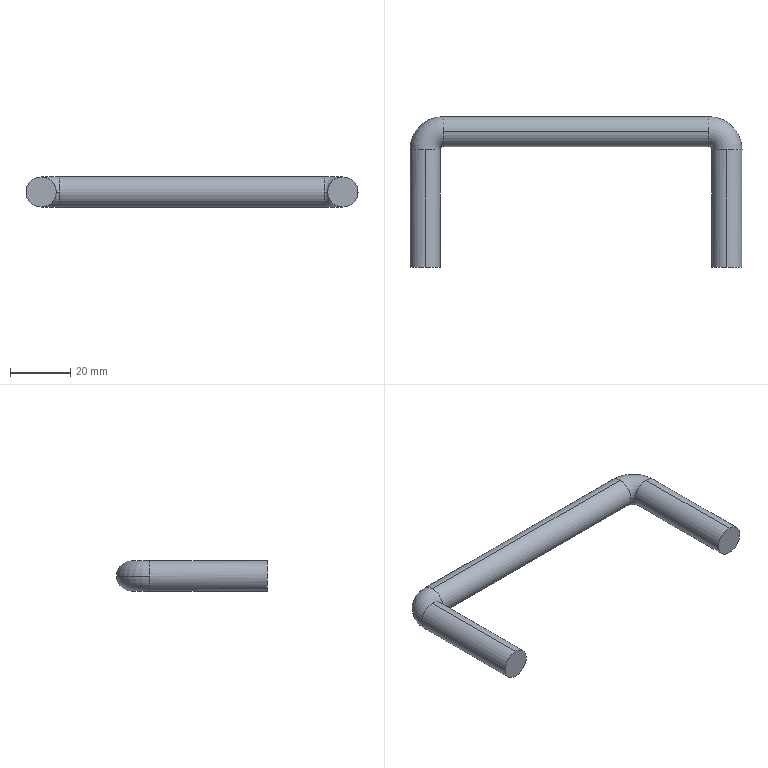Part | SolidWorks | features Sweep 1 | 1 solid | 12 faces | box 110 x 50 x 10 mm | volume 14518 mm3 | cylinder 6 | torus 4 | plane 2 | commonest cylinder face diameters 10 x6
STEP:
#1=CARTESIAN_POINT('',(-15.998,28.558,-5.));
#2=VERTEX_POINT('',#1);
#3=CARTESIAN_POINT('',(-20.998,28.558,0.));
#4=VERTEX_POINT('',#3);
#5=CARTESIAN_POINT('',(-15.998,28.558,0.));
#6=DIRECTION('',(0.,1.,0.));
#7=DIRECTION('',(0.,0.,1.));
#8=AXIS2_PLACEMENT_3D('',#5,#6,#7);
#9=CIRCLE('',#8,5.);
#10=EDGE_CURVE('',#2,#4,#9,.T.);
#11=ORIENTED_EDGE('',*,*,#10,.T.);
#12=CARTESIAN_POINT('',(-9.998,39.558,0.));
#13=VERTEX_POINT('',#12);
#14=CARTESIAN_POINT('',(-9.998,28.558,0.));
#15=DIRECTION('',(0.,0.,-1.));
#16=DIRECTION('',(-1.,0.,0.));
#17=AXIS2_PLACEMENT_3D('',#14,#15,#16);
#18=CIRCLE('',#17,11.);
#19=EDGE_CURVE('',#4,#13,#18,.T.);
#20=ORIENTED_EDGE('',*,*,#19,.T.);
#21=CARTESIAN_POINT('',(-9.998,34.558,-5.));
#22=VERTEX_POINT('',#21);
#23=CARTESIAN_POINT('',(-9.998,34.558,0.));
#24=DIRECTION('',(1.,0.,0.));
#25=DIRECTION('',(0.,0.,1.));
#26=AXIS2_PLACEMENT_3D('',#23,#24,#25);
#27=CIRCLE('',#26,5.);
#28=EDGE_CURVE('',#22,#13,#27,.T.);
#29=ORIENTED_EDGE('',*,*,#28,.F.);
#30=CARTESIAN_POINT('',(-9.998,29.558,0.));
#31=VERTEX_POINT('',#30);
#32=CARTESIAN_POINT('',(-9.998,34.558,0.));
#33=DIRECTION('',(1.,0.,0.));
#34=DIRECTION('',(0.,0.,1.));
#35=AXIS2_PLACEMENT_3D('',#32,#33,#34);
#36=CIRCLE('',#35,5.);
#37=EDGE_CURVE('',#31,#22,#36,.T.);
#38=ORIENTED_EDGE('',*,*,#37,.F.);
#39=CARTESIAN_POINT('',(-10.998,28.558,0.));
#40=VERTEX_POINT('',#39);
#41=CARTESIAN_POINT('',(-9.998,28.558,0.));
#42=DIRECTION('',(0.,0.,-1.));
#43=DIRECTION('',(-1.,0.,0.));
#44=AXIS2_PLACEMENT_3D('',#41,#42,#43);
#45=CIRCLE('',#44,1.);
#46=EDGE_CURVE('',#40,#31,#45,.T.);
#47=ORIENTED_EDGE('',*,*,#46,.F.);
#48=CARTESIAN_POINT('',(-15.998,28.558,0.));
#49=DIRECTION('',(0.,1.,0.));
#50=DIRECTION('',(0.,0.,1.));
#51=AXIS2_PLACEMENT_3D('',#48,#49,#50);
#52=CIRCLE('',#51,5.);
#53=EDGE_CURVE('',#40,#2,#52,.T.);
#54=ORIENTED_EDGE('',*,*,#53,.T.);
#55=EDGE_LOOP('',(#11,#20,#29,#38,#47,#54));
#56=FACE_OUTER_BOUND('',#55,.T.);
#57=CARTESIAN_POINT('',(-9.998,28.558,0.));
#58=DIRECTION('',(0.,0.,-1.));
#59=DIRECTION('',(-1.,0.,0.));
#60=AXIS2_PLACEMENT_3D('',#57,#58,#59);
#61=TOROIDAL_SURFACE('',#60,6.,5.);
#62=ADVANCED_FACE('',(#56),#61,.T.);
#63=CARTESIAN_POINT('',(78.002,34.558,-5.));
#64=VERTEX_POINT('',#63);
#65=CARTESIAN_POINT('',(78.002,39.558,0.));
#66=VERTEX_POINT('',#65);
#67=CARTESIAN_POINT('',(78.002,34.558,0.));
#68=DIRECTION('',(1.,0.,0.));
#69=DIRECTION('',(0.,0.,1.));
#70=AXIS2_PLACEMENT_3D('',#67,#68,#69);
#71=CIRCLE('',#70,5.);
#72=EDGE_CURVE('',#64,#66,#71,.T.);
#73=ORIENTED_EDGE('',*,*,#72,.T.);
#74=CARTESIAN_POINT('',(89.002,28.558,0.));
#75=VERTEX_POINT('',#74);
#76=CARTESIAN_POINT('',(78.002,28.558,0.));
#77=DIRECTION('',(0.,0.,-1.));
#78=DIRECTION('',(-1.,0.,0.));
#79=AXIS2_PLACEMENT_3D('',#76,#77,#78);
#80=CIRCLE('',#79,11.);
#81=EDGE_CURVE('',#66,#75,#80,.T.);
#82=ORIENTED_EDGE('',*,*,#81,.T.);
#83=CARTESIAN_POINT('',(84.002,28.558,-5.));
#84=VERTEX_POINT('',#83);
#85=CARTESIAN_POINT('',(84.002,28.558,0.));
#86=DIRECTION('',(0.,-1.,0.));
#87=DIRECTION('',(0.,0.,1.));
#88=AXIS2_PLACEMENT_3D('',#85,#86,#87);
#89=CIRCLE('',#88,5.);
#90=EDGE_CURVE('',#84,#75,#89,.T.);
#91=ORIENTED_EDGE('',*,*,#90,.F.);
#92=CARTESIAN_POINT('',(79.002,28.558,0.));
#93=VERTEX_POINT('',#92);
#94=CARTESIAN_POINT('',(84.002,28.558,0.));
#95=DIRECTION('',(0.,-1.,0.));
#96=DIRECTION('',(0.,0.,1.));
#97=AXIS2_PLACEMENT_3D('',#94,#95,#96);
#98=CIRCLE('',#97,5.);
#99=EDGE_CURVE('',#93,#84,#98,.T.);
#100=ORIENTED_EDGE('',*,*,#99,.F.);
#101=CARTESIAN_POINT('',(78.002,29.558,0.));
#102=VERTEX_POINT('',#101);
#103=CARTESIAN_POINT('',(78.002,28.558,0.));
#104=DIRECTION('',(0.,0.,-1.));
#105=DIRECTION('',(-1.,0.,0.));
#106=AXIS2_PLACEMENT_3D('',#103,#104,#105);
#107=CIRCLE('',#106,1.);
#108=EDGE_CURVE('',#102,#93,#107,.T.);
#109=ORIENTED_EDGE('',*,*,#108,.F.);
#110=CARTESIAN_POINT('',(78.002,34.558,0.));
#111=DIRECTION('',(1.,0.,0.));
#112=DIRECTION('',(0.,0.,1.));
#113=AXIS2_PLACEMENT_3D('',#110,#111,#112);
#114=CIRCLE('',#113,5.);
#115=EDGE_CURVE('',#102,#64,#114,.T.);
#116=ORIENTED_EDGE('',*,*,#115,.T.);
#117=EDGE_LOOP('',(#73,#82,#91,#100,#109,#116));
#118=FACE_OUTER_BOUND('',#117,.T.);
#119=CARTESIAN_POINT('',(78.002,28.558,0.));
#120=DIRECTION('',(0.,0.,-1.));
#121=DIRECTION('',(-1.,0.,0.));
#122=AXIS2_PLACEMENT_3D('',#119,#120,#121);
#123=TOROIDAL_SURFACE('',#122,6.,5.);
#124=ADVANCED_FACE('',(#118),#123,.T.);
#125=CARTESIAN_POINT('',(-15.998,28.558,5.));
#126=VERTEX_POINT('',#125);
#127=CARTESIAN_POINT('',(-15.998,28.558,0.));
#128=DIRECTION('',(0.,1.,0.));
#129=DIRECTION('',(0.,0.,1.));
#130=AXIS2_PLACEMENT_3D('',#127,#128,#129);
#131=CIRCLE('',#130,5.);
#132=EDGE_CURVE('',#126,#40,#131,.T.);
#133=ORIENTED_EDGE('',*,*,#132,.F.);
#134=CARTESIAN_POINT('',(-15.998,-10.442,5.));
#135=VERTEX_POINT('',#134);
#136=CARTESIAN_POINT('',(-15.998,28.558,5.));
#137=DIRECTION('',(0.,-1.,0.));
#138=VECTOR('',#137,1000.);
#139=LINE('',#136,#138);
#140=EDGE_CURVE('',#126,#135,#139,.T.);
#141=ORIENTED_EDGE('',*,*,#140,.T.);
#142=CARTESIAN_POINT('',(-15.998,-10.442,-5.));
#143=VERTEX_POINT('',#142);
#144=CARTESIAN_POINT('',(-15.998,-10.442,0.));
#145=DIRECTION('',(0.,1.,0.));
#146=DIRECTION('',(0.,0.,1.));
#147=AXIS2_PLACEMENT_3D('',#144,#145,#146);
#148=CIRCLE('',#147,5.);
#149=EDGE_CURVE('',#135,#143,#148,.T.);
#150=ORIENTED_EDGE('',*,*,#149,.T.);
#151=CARTESIAN_POINT('',(-15.998,28.558,-5.));
#152=DIRECTION('',(0.,-1.,0.));
#153=VECTOR('',#152,1000.);
#154=LINE('',#151,#153);
#155=EDGE_CURVE('',#2,#143,#154,.T.);
#156=ORIENTED_EDGE('',*,*,#155,.F.);
#157=ORIENTED_EDGE('',*,*,#53,.F.);
#158=EDGE_LOOP('',(#133,#141,#150,#156,#157));
#159=FACE_OUTER_BOUND('',#158,.T.);
#160=CARTESIAN_POINT('',(-15.998,28.558,0.));
#161=DIRECTION('',(0.,-1.,0.));
#162=DIRECTION('',(0.,0.,-1.));
#163=AXIS2_PLACEMENT_3D('',#160,#161,#162);
#164=CYLINDRICAL_SURFACE('',#163,5.);
#165=ADVANCED_FACE('',(#159),#164,.T.);
#166=ORIENTED_EDGE('',*,*,#28,.T.);
#167=CARTESIAN_POINT('',(-9.998,34.558,5.));
#168=VERTEX_POINT('',#167);
#169=CARTESIAN_POINT('',(-9.998,34.558,0.));
#170=DIRECTION('',(1.,0.,0.));
#171=DIRECTION('',(0.,0.,1.));
#172=AXIS2_PLACEMENT_3D('',#169,#170,#171);
#173=CIRCLE('',#172,5.);
#174=EDGE_CURVE('',#13,#168,#173,.T.);
#175=ORIENTED_EDGE('',*,*,#174,.T.);
#176=CARTESIAN_POINT('',(78.002,34.558,5.));
#177=VERTEX_POINT('',#176);
#178=CARTESIAN_POINT('',(-9.998,34.558,5.));
#179=DIRECTION('',(1.,0.,0.));
#180=VECTOR('',#179,1000.);
#181=LINE('',#178,#180);
#182=EDGE_CURVE('',#168,#177,#181,.T.);
#183=ORIENTED_EDGE('',*,*,#182,.T.);
#184=CARTESIAN_POINT('',(78.002,34.558,0.));
#185=DIRECTION('',(1.,0.,0.));
#186=DIRECTION('',(0.,0.,1.));
#187=AXIS2_PLACEMENT_3D('',#184,#185,#186);
#188=CIRCLE('',#187,5.);
#189=EDGE_CURVE('',#66,#177,#188,.T.);
#190=ORIENTED_EDGE('',*,*,#189,.F.);
#191=ORIENTED_EDGE('',*,*,#72,.F.);
#192=CARTESIAN_POINT('',(-9.998,34.558,-5.));
#193=DIRECTION('',(1.,0.,0.));
#194=VECTOR('',#193,1000.);
#195=LINE('',#192,#194);
#196=EDGE_CURVE('',#22,#64,#195,.T.);
#197=ORIENTED_EDGE('',*,*,#196,.F.);
#198=EDGE_LOOP('',(#166,#175,#183,#190,#191,#197));
#199=FACE_OUTER_BOUND('',#198,.T.);
#200=CARTESIAN_POINT('',(-9.998,34.558,0.));
#201=DIRECTION('',(1.,0.,0.));
#202=DIRECTION('',(0.,0.,-1.));
#203=AXIS2_PLACEMENT_3D('',#200,#201,#202);
#204=CYLINDRICAL_SURFACE('',#203,5.);
#205=ADVANCED_FACE('',(#199),#204,.T.);
#206=ORIENTED_EDGE('',*,*,#90,.T.);
#207=CARTESIAN_POINT('',(84.002,28.558,5.));
#208=VERTEX_POINT('',#207);
#209=CARTESIAN_POINT('',(84.002,28.558,0.));
#210=DIRECTION('',(0.,-1.,0.));
#211=DIRECTION('',(0.,0.,1.));
#212=AXIS2_PLACEMENT_3D('',#209,#210,#211);
#213=CIRCLE('',#212,5.);
#214=EDGE_CURVE('',#75,#208,#213,.T.);
#215=ORIENTED_EDGE('',*,*,#214,.T.);
#216=CARTESIAN_POINT('',(84.002,-10.442,5.));
#217=VERTEX_POINT('',#216);
#218=CARTESIAN_POINT('',(84.002,28.558,5.));
#219=DIRECTION('',(0.,-1.,0.));
#220=VECTOR('',#219,1000.);
#221=LINE('',#218,#220);
#222=EDGE_CURVE('',#208,#217,#221,.T.);
#223=ORIENTED_EDGE('',*,*,#222,.T.);
#224=CARTESIAN_POINT('',(84.002,-10.442,-5.));
#225=VERTEX_POINT('',#224);
#226=CARTESIAN_POINT('',(84.002,-10.442,0.));
#227=DIRECTION('',(0.,-1.,0.));
#228=DIRECTION('',(0.,0.,1.));
#229=AXIS2_PLACEMENT_3D('',#226,#227,#228);
#230=CIRCLE('',#229,5.);
#231=EDGE_CURVE('',#225,#217,#230,.T.);
#232=ORIENTED_EDGE('',*,*,#231,.F.);
#233=CARTESIAN_POINT('',(84.002,28.558,-5.));
#234=DIRECTION('',(0.,-1.,0.));
#235=VECTOR('',#234,1000.);
#236=LINE('',#233,#235);
#237=EDGE_CURVE('',#84,#225,#236,.T.);
#238=ORIENTED_EDGE('',*,*,#237,.F.);
#239=EDGE_LOOP('',(#206,#215,#223,#232,#238));
#240=FACE_OUTER_BOUND('',#239,.T.);
#241=CARTESIAN_POINT('',(84.002,28.558,0.));
#242=DIRECTION('',(0.,-1.,0.));
#243=DIRECTION('',(0.,0.,-1.));
#244=AXIS2_PLACEMENT_3D('',#241,#242,#243);
#245=CYLINDRICAL_SURFACE('',#244,5.);
#246=ADVANCED_FACE('',(#240),#245,.T.);
#247=ORIENTED_EDGE('',*,*,#222,.F.);
#248=CARTESIAN_POINT('',(84.002,28.558,0.));
#249=DIRECTION('',(0.,-1.,0.));
#250=DIRECTION('',(0.,0.,1.));
#251=AXIS2_PLACEMENT_3D('',#248,#249,#250);
#252=CIRCLE('',#251,5.);
#253=EDGE_CURVE('',#208,#93,#252,.T.);
#254=ORIENTED_EDGE('',*,*,#253,.T.);
#255=ORIENTED_EDGE('',*,*,#99,.T.);
#256=ORIENTED_EDGE('',*,*,#237,.T.);
#257=CARTESIAN_POINT('',(84.002,-10.442,0.));
#258=DIRECTION('',(0.,-1.,0.));
#259=DIRECTION('',(0.,0.,1.));
#260=AXIS2_PLACEMENT_3D('',#257,#258,#259);
#261=CIRCLE('',#260,5.);
#262=EDGE_CURVE('',#217,#225,#261,.T.);
#263=ORIENTED_EDGE('',*,*,#262,.F.);
#264=EDGE_LOOP('',(#247,#254,#255,#256,#263));
#265=FACE_OUTER_BOUND('',#264,.T.);
#266=CARTESIAN_POINT('',(84.002,28.558,0.));
#267=DIRECTION('',(0.,-1.,0.));
#268=DIRECTION('',(0.,0.,-1.));
#269=AXIS2_PLACEMENT_3D('',#266,#267,#268);
#270=CYLINDRICAL_SURFACE('',#269,5.);
#271=ADVANCED_FACE('',(#265),#270,.T.);
#272=ORIENTED_EDGE('',*,*,#81,.F.);
#273=ORIENTED_EDGE('',*,*,#189,.T.);
#274=CARTESIAN_POINT('',(78.002,34.558,0.));
#275=DIRECTION('',(1.,0.,0.));
#276=DIRECTION('',(0.,0.,1.));
#277=AXIS2_PLACEMENT_3D('',#274,#275,#276);
#278=CIRCLE('',#277,5.);
#279=EDGE_CURVE('',#177,#102,#278,.T.);
#280=ORIENTED_EDGE('',*,*,#279,.T.);
#281=ORIENTED_EDGE('',*,*,#108,.T.);
#282=ORIENTED_EDGE('',*,*,#253,.F.);
#283=ORIENTED_EDGE('',*,*,#214,.F.);
#284=EDGE_LOOP('',(#272,#273,#280,#281,#282,#283));
#285=FACE_OUTER_BOUND('',#284,.T.);
#286=CARTESIAN_POINT('',(78.002,28.558,0.));
#287=DIRECTION('',(0.,0.,-1.));
#288=DIRECTION('',(-1.,0.,0.));
#289=AXIS2_PLACEMENT_3D('',#286,#287,#288);
#290=TOROIDAL_SURFACE('',#289,6.,5.);
#291=ADVANCED_FACE('',(#285),#290,.T.);
#292=ORIENTED_EDGE('',*,*,#182,.F.);
#293=CARTESIAN_POINT('',(-9.998,34.558,0.));
#294=DIRECTION('',(1.,0.,0.));
#295=DIRECTION('',(0.,0.,1.));
#296=AXIS2_PLACEMENT_3D('',#293,#294,#295);
#297=CIRCLE('',#296,5.);
#298=EDGE_CURVE('',#168,#31,#297,.T.);
#299=ORIENTED_EDGE('',*,*,#298,.T.);
#300=ORIENTED_EDGE('',*,*,#37,.T.);
#301=ORIENTED_EDGE('',*,*,#196,.T.);
#302=ORIENTED_EDGE('',*,*,#115,.F.);
#303=ORIENTED_EDGE('',*,*,#279,.F.);
#304=EDGE_LOOP('',(#292,#299,#300,#301,#302,#303));
#305=FACE_OUTER_BOUND('',#304,.T.);
#306=CARTESIAN_POINT('',(-9.998,34.558,0.));
#307=DIRECTION('',(1.,0.,0.));
#308=DIRECTION('',(0.,0.,-1.));
#309=AXIS2_PLACEMENT_3D('',#306,#307,#308);
#310=CYLINDRICAL_SURFACE('',#309,5.);
#311=ADVANCED_FACE('',(#305),#310,.T.);
#312=ORIENTED_EDGE('',*,*,#19,.F.);
#313=CARTESIAN_POINT('',(-15.998,28.558,0.));
#314=DIRECTION('',(0.,1.,0.));
#315=DIRECTION('',(0.,0.,1.));
#316=AXIS2_PLACEMENT_3D('',#313,#314,#315);
#317=CIRCLE('',#316,5.);
#318=EDGE_CURVE('',#4,#126,#317,.T.);
#319=ORIENTED_EDGE('',*,*,#318,.T.);
#320=ORIENTED_EDGE('',*,*,#132,.T.);
#321=ORIENTED_EDGE('',*,*,#46,.T.);
#322=ORIENTED_EDGE('',*,*,#298,.F.);
#323=ORIENTED_EDGE('',*,*,#174,.F.);
#324=EDGE_LOOP('',(#312,#319,#320,#321,#322,#323));
#325=FACE_OUTER_BOUND('',#324,.T.);
#326=CARTESIAN_POINT('',(-9.998,28.558,0.));
#327=DIRECTION('',(0.,0.,-1.));
#328=DIRECTION('',(-1.,0.,0.));
#329=AXIS2_PLACEMENT_3D('',#326,#327,#328);
#330=TOROIDAL_SURFACE('',#329,6.,5.);
#331=ADVANCED_FACE('',(#325),#330,.T.);
#332=ORIENTED_EDGE('',*,*,#140,.F.);
#333=ORIENTED_EDGE('',*,*,#318,.F.);
#334=ORIENTED_EDGE('',*,*,#10,.F.);
#335=ORIENTED_EDGE('',*,*,#155,.T.);
#336=CARTESIAN_POINT('',(-15.998,-10.442,0.));
#337=DIRECTION('',(0.,1.,0.));
#338=DIRECTION('',(0.,0.,1.));
#339=AXIS2_PLACEMENT_3D('',#336,#337,#338);
#340=CIRCLE('',#339,5.);
#341=EDGE_CURVE('',#143,#135,#340,.T.);
#342=ORIENTED_EDGE('',*,*,#341,.T.);
#343=EDGE_LOOP('',(#332,#333,#334,#335,#342));
#344=FACE_OUTER_BOUND('',#343,.T.);
#345=CARTESIAN_POINT('',(-15.998,28.558,0.));
#346=DIRECTION('',(0.,-1.,0.));
#347=DIRECTION('',(0.,0.,-1.));
#348=AXIS2_PLACEMENT_3D('',#345,#346,#347);
#349=CYLINDRICAL_SURFACE('',#348,5.);
#350=ADVANCED_FACE('',(#344),#349,.T.);
#351=ORIENTED_EDGE('',*,*,#231,.T.);
#352=ORIENTED_EDGE('',*,*,#262,.T.);
#353=EDGE_LOOP('',(#351,#352));
#354=FACE_OUTER_BOUND('',#353,.T.);
#355=CARTESIAN_POINT('',(84.002,-10.442,0.));
#356=DIRECTION('',(0.,-1.,0.));
#357=DIRECTION('',(0.,0.,1.));
#358=AXIS2_PLACEMENT_3D('',#355,#356,#357);
#359=PLANE('',#358);
#360=ADVANCED_FACE('',(#354),#359,.T.);
#361=ORIENTED_EDGE('',*,*,#341,.F.);
#362=ORIENTED_EDGE('',*,*,#149,.F.);
#363=EDGE_LOOP('',(#361,#362));
#364=FACE_OUTER_BOUND('',#363,.T.);
#365=CARTESIAN_POINT('',(-15.998,-10.442,0.));
#366=DIRECTION('',(0.,1.,0.));
#367=DIRECTION('',(0.,0.,1.));
#368=AXIS2_PLACEMENT_3D('',#365,#366,#367);
#369=PLANE('',#368);
#370=ADVANCED_FACE('',(#364),#369,.F.);
#371=CLOSED_SHELL('',(#62,#124,#165,#205,#246,#271,#291,#311,#331,#350,#360,#370));
#372=MANIFOLD_SOLID_BREP('',#371);
#373=CARTESIAN_POINT('',(0.,0.,0.));
#374=DIRECTION('',(0.,0.,1.));
#375=DIRECTION('',(1.,0.,0.));
#376=AXIS2_PLACEMENT_3D('',#373,#374,#375);
#377=(LENGTH_UNIT()NAMED_UNIT(*)SI_UNIT(.MILLI.,.METRE.));
#378=UNCERTAINTY_MEASURE_WITH_UNIT(LENGTH_MEASURE(0.00001),#377,'','');
#379=(NAMED_UNIT(*)PLANE_ANGLE_UNIT()SI_UNIT($,.RADIAN.));
#380=(NAMED_UNIT(*)SI_UNIT($,.STERADIAN.)SOLID_ANGLE_UNIT());
#381=(GEOMETRIC_REPRESENTATION_CONTEXT(3)GLOBAL_UNCERTAINTY_ASSIGNED_CONTEXT((#378))GLOBAL_UNIT_ASSIGNED_CONTEXT((#377,#379,#380))REPRESENTATION_CONTEXT('',''));
#382=ADVANCED_BREP_SHAPE_REPRESENTATION('',(#372,#376),#381);